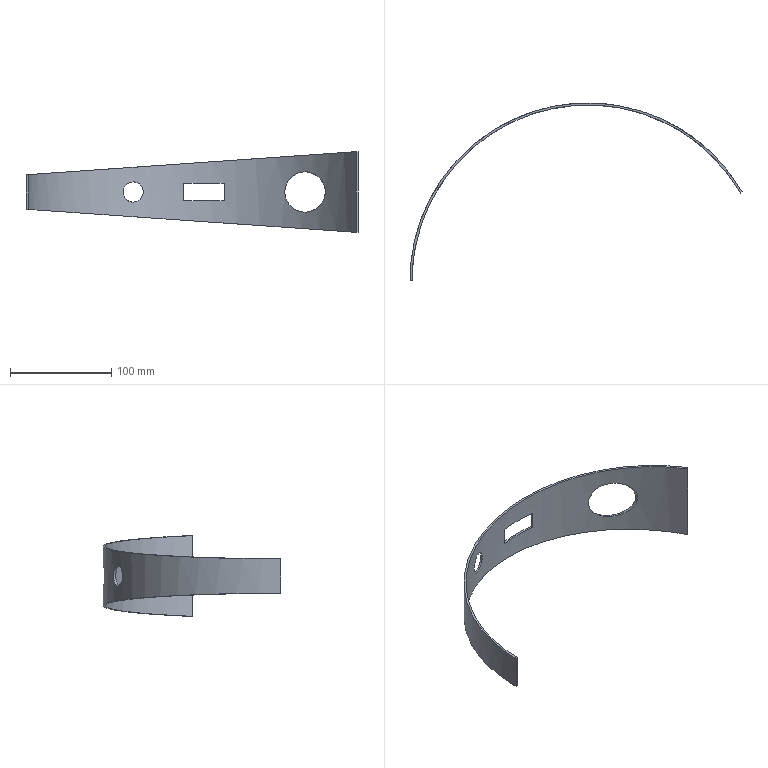Part | SolidWorks | features ICE 4, ExtruRefSurface 1, Thicken 1 | 1 solid | 14 faces | box 328.42 x 176 x 80 mm | volume 44356 mm3 | plane 8 | cylinder 6 | commonest cylinder face diameters 20 x2 40 x2 348 x1 352 x1
STEP:
#1=CARTESIAN_POINT('',(-70.,161.481,-10.));
#2=VERTEX_POINT('',#1);
#3=CARTESIAN_POINT('',(-70.,161.481,10.));
#4=VERTEX_POINT('',#3);
#5=CARTESIAN_POINT('',(-70.,161.481,-10.));
#6=CARTESIAN_POINT('',(-70.637,161.205,-10.));
#7=CARTESIAN_POINT('',(-71.263,160.929,-9.94));
#8=CARTESIAN_POINT('',(-72.494,160.378,-9.704));
#9=CARTESIAN_POINT('',(-73.101,160.102,-9.528));
#10=CARTESIAN_POINT('',(-74.285,159.556,-9.058));
#11=CARTESIAN_POINT('',(-74.849,159.292,-8.769));
#12=CARTESIAN_POINT('',(-75.652,158.912,-8.256));
#13=CARTESIAN_POINT('',(-75.912,158.787,-8.072));
#14=CARTESIAN_POINT('',(-76.419,158.544,-7.675));
#15=CARTESIAN_POINT('',(-76.666,158.425,-7.461));
#16=CARTESIAN_POINT('',(-77.375,158.08,-6.785));
#17=CARTESIAN_POINT('',(-77.8,157.871,-6.292));
#18=CARTESIAN_POINT('',(-78.368,157.59,-5.485));
#19=CARTESIAN_POINT('',(-78.545,157.502,-5.205));
#20=CARTESIAN_POINT('',(-78.874,157.337,-4.622));
#21=CARTESIAN_POINT('',(-79.027,157.26,-4.317));
#22=CARTESIAN_POINT('',(-79.433,157.056,-3.387));
#23=CARTESIAN_POINT('',(-79.64,156.95,-2.744));
#24=CARTESIAN_POINT('',(-79.853,156.842,-1.742));
#25=CARTESIAN_POINT('',(-79.908,156.814,-1.4));
#26=CARTESIAN_POINT('',(-79.981,156.777,-0.7103));
#27=CARTESIAN_POINT('',(-79.999,156.768,-0.3661));
#28=CARTESIAN_POINT('',(-80.002,156.767,0.6638));
#29=CARTESIAN_POINT('',(-79.933,156.802,1.349));
#30=CARTESIAN_POINT('',(-79.652,156.944,2.704));
#31=CARTESIAN_POINT('',(-79.446,157.049,3.352));
#32=CARTESIAN_POINT('',(-79.043,157.252,4.282));
#33=CARTESIAN_POINT('',(-78.893,157.328,4.586));
#34=CARTESIAN_POINT('',(-78.564,157.492,5.174));
#35=CARTESIAN_POINT('',(-78.386,157.58,5.457));
#36=CARTESIAN_POINT('',(-78.007,157.768,5.999));
#37=CARTESIAN_POINT('',(-77.806,157.868,6.259));
#38=CARTESIAN_POINT('',(-77.378,158.078,6.758));
#39=CARTESIAN_POINT('',(-77.152,158.189,6.997));
#40=CARTESIAN_POINT('',(-76.443,158.533,7.676));
#41=CARTESIAN_POINT('',(-75.936,158.777,8.073));
#42=CARTESIAN_POINT('',(-75.13,159.159,8.59));
#43=CARTESIAN_POINT('',(-74.853,159.29,8.749));
#44=CARTESIAN_POINT('',(-74.283,159.556,9.042));
#45=CARTESIAN_POINT('',(-73.992,159.691,9.174));
#46=CARTESIAN_POINT('',(-73.11,160.098,9.525));
#47=CARTESIAN_POINT('',(-72.506,160.373,9.701));
#48=CARTESIAN_POINT('',(-71.268,160.927,9.939));
#49=CARTESIAN_POINT('',(-70.63,161.208,10.));
#50=CARTESIAN_POINT('',(-70.,161.481,10.));
#51=B_SPLINE_CURVE_WITH_KNOTS('',3,(#5,#6,#7,#8,#9,#10,#11,#12,#13,#14,#15,#16,#17,#18,#19,#20,#21,#22,#23,#24,#25,#26,#27,#28,#29,#30,#31,#32,#33,#34,#35,#36,#37,#38,#39,#40,#41,#42,#43,#44,#45,#46,#47,#48,#49,#50),.UNSPECIFIED.,.F.,.F.,(4,2,2,2,2,2,2,2,2,2,2,2,2,2,2,2,2,2,2,2,2,2,4),(0.,0.002054,0.004107,0.006161,0.007188,0.008214,0.01027,0.01129,0.01232,0.01438,0.0154,0.01643,0.01848,0.02054,0.02156,0.02259,0.02362,0.02464,0.0267,0.02772,0.02875,0.0308,0.03286),.UNSPECIFIED.);
#52=EDGE_CURVE('',#2,#4,#51,.T.);
#53=ORIENTED_EDGE('',*,*,#52,.T.);
#54=CARTESIAN_POINT('',(-70.,159.298,10.));
#55=VERTEX_POINT('',#54);
#56=CARTESIAN_POINT('',(-70.,176.001,10.));
#57=DIRECTION('',(0.,-1.,0.));
#58=VECTOR('',#57,1000.);
#59=LINE('',#56,#58);
#60=EDGE_CURVE('',#4,#55,#59,.T.);
#61=ORIENTED_EDGE('',*,*,#60,.T.);
#62=CARTESIAN_POINT('',(-70.,159.298,-10.));
#63=VERTEX_POINT('',#62);
#64=CARTESIAN_POINT('',(-70.,159.298,10.));
#65=CARTESIAN_POINT('',(-70.629,159.022,10.));
#66=CARTESIAN_POINT('',(-71.253,158.743,9.941));
#67=CARTESIAN_POINT('',(-72.183,158.322,9.764));
#68=CARTESIAN_POINT('',(-72.493,158.18,9.69));
#69=CARTESIAN_POINT('',(-73.099,157.901,9.513));
#70=CARTESIAN_POINT('',(-73.397,157.763,9.411));
#71=CARTESIAN_POINT('',(-74.273,157.353,9.063));
#72=CARTESIAN_POINT('',(-74.836,157.086,8.776));
#73=CARTESIAN_POINT('',(-75.646,156.696,8.26));
#74=CARTESIAN_POINT('',(-75.911,156.568,8.072));
#75=CARTESIAN_POINT('',(-76.418,156.321,7.675));
#76=CARTESIAN_POINT('',(-76.662,156.202,7.465));
#77=CARTESIAN_POINT('',(-77.362,155.857,6.798));
#78=CARTESIAN_POINT('',(-77.789,155.644,6.307));
#79=CARTESIAN_POINT('',(-78.364,155.355,5.491));
#80=CARTESIAN_POINT('',(-78.544,155.264,5.206));
#81=CARTESIAN_POINT('',(-78.873,155.097,4.624));
#82=CARTESIAN_POINT('',(-79.022,155.021,4.326));
#83=CARTESIAN_POINT('',(-79.292,154.883,3.712));
#84=CARTESIAN_POINT('',(-79.411,154.822,3.397));
#85=CARTESIAN_POINT('',(-79.62,154.715,2.751));
#86=CARTESIAN_POINT('',(-79.71,154.669,2.417));
#87=CARTESIAN_POINT('',(-79.925,154.557,1.404));
#88=CARTESIAN_POINT('',(-79.998,154.52,0.7221));
#89=CARTESIAN_POINT('',(-80.001,154.518,-0.3097));
#90=CARTESIAN_POINT('',(-79.984,154.527,-0.6562));
#91=CARTESIAN_POINT('',(-79.915,154.563,-1.348));
#92=CARTESIAN_POINT('',(-79.862,154.59,-1.688));
#93=CARTESIAN_POINT('',(-79.724,154.661,-2.359));
#94=CARTESIAN_POINT('',(-79.638,154.706,-2.689));
#95=CARTESIAN_POINT('',(-79.432,154.811,-3.339));
#96=CARTESIAN_POINT('',(-79.313,154.873,-3.66));
#97=CARTESIAN_POINT('',(-78.907,155.08,-4.597));
#98=CARTESIAN_POINT('',(-78.58,155.246,-5.18));
#99=CARTESIAN_POINT('',(-78.01,155.533,-5.996));
#100=CARTESIAN_POINT('',(-77.806,155.635,-6.259));
#101=CARTESIAN_POINT('',(-77.376,155.849,-6.76));
#102=CARTESIAN_POINT('',(-77.151,155.961,-6.997));
#103=CARTESIAN_POINT('',(-76.449,156.307,-7.67));
#104=CARTESIAN_POINT('',(-75.943,156.554,-8.068));
#105=CARTESIAN_POINT('',(-74.857,157.076,-8.765));
#106=CARTESIAN_POINT('',(-74.292,157.344,-9.054));
#107=CARTESIAN_POINT('',(-73.414,157.755,-9.405));
#108=CARTESIAN_POINT('',(-73.116,157.893,-9.508));
#109=CARTESIAN_POINT('',(-72.509,158.173,-9.685));
#110=CARTESIAN_POINT('',(-72.199,158.314,-9.76));
#111=CARTESIAN_POINT('',(-71.266,158.737,-9.94));
#112=CARTESIAN_POINT('',(-70.636,159.019,-10.));
#113=CARTESIAN_POINT('',(-70.,159.298,-10.));
#114=B_SPLINE_CURVE_WITH_KNOTS('',3,(#64,#65,#66,#67,#68,#69,#70,#71,#72,#73,#74,#75,#76,#77,#78,#79,#80,#81,#82,#83,#84,#85,#86,#87,#88,#89,#90,#91,#92,#93,#94,#95,#96,#97,#98,#99,#100,#101,#102,#103,#104,#105,#106,#107,#108,#109,#110,#111,#112,#113),.UNSPECIFIED.,.F.,.F.,(4,2,2,2,2,2,2,2,2,2,2,2,2,2,2,2,2,2,2,2,2,2,2,2,4),(0.0325,0.03456,0.03558,0.03661,0.03867,0.0397,0.04072,0.04278,0.04381,0.04483,0.04586,0.04689,0.04895,0.04997,0.051,0.05203,0.05306,0.05511,0.05614,0.05717,0.05922,0.06128,0.06231,0.06334,0.06539),.UNSPECIFIED.);
#115=EDGE_CURVE('',#55,#63,#114,.T.);
#116=ORIENTED_EDGE('',*,*,#115,.T.);
#117=CARTESIAN_POINT('',(-70.,176.001,-10.));
#118=DIRECTION('',(0.,-1.,0.));
#119=VECTOR('',#118,1000.);
#120=LINE('',#117,#119);
#121=EDGE_CURVE('',#2,#63,#120,.T.);
#122=ORIENTED_EDGE('',*,*,#121,.F.);
#123=EDGE_LOOP('',(#53,#61,#116,#122));
#124=FACE_OUTER_BOUND('',#123,.T.);
#125=CARTESIAN_POINT('',(-70.,176.001,0.));
#126=DIRECTION('',(0.,-1.,0.));
#127=DIRECTION('',(0.,0.,-1.));
#128=AXIS2_PLACEMENT_3D('',#125,#126,#127);
#129=CYLINDRICAL_SURFACE('',#128,10.);
#130=ADVANCED_FACE('',(#124),#129,.F.);
#131=CARTESIAN_POINT('',(100.,144.831,-20.));
#132=VERTEX_POINT('',#131);
#133=CARTESIAN_POINT('',(100.,144.831,20.));
#134=VERTEX_POINT('',#133);
#135=CARTESIAN_POINT('',(100.,144.831,-20.));
#136=CARTESIAN_POINT('',(98.822,145.645,-20.));
#137=CARTESIAN_POINT('',(97.649,146.433,-19.897));
#138=CARTESIAN_POINT('',(95.319,147.96,-19.48));
#139=CARTESIAN_POINT('',(94.161,148.699,-19.168));
#140=CARTESIAN_POINT('',(92.726,149.593,-18.633));
#141=CARTESIAN_POINT('',(92.439,149.77,-18.518));
#142=CARTESIAN_POINT('',(91.867,150.122,-18.274));
#143=CARTESIAN_POINT('',(91.581,150.296,-18.145));
#144=CARTESIAN_POINT('',(90.733,150.811,-17.735));
#145=CARTESIAN_POINT('',(90.179,151.142,-17.434));
#146=CARTESIAN_POINT('',(88.556,152.103,-16.451));
#147=CARTESIAN_POINT('',(87.522,152.699,-15.686));
#148=CARTESIAN_POINT('',(86.059,153.526,-14.356));
#149=CARTESIAN_POINT('',(85.585,153.79,-13.88));
#150=CARTESIAN_POINT('',(84.693,154.284,-12.889));
#151=CARTESIAN_POINT('',(84.27,154.515,-12.37));
#152=CARTESIAN_POINT('',(83.475,154.946,-11.286));
#153=CARTESIAN_POINT('',(83.102,155.146,-10.721));
#154=CARTESIAN_POINT('',(82.409,155.515,-9.541));
#155=CARTESIAN_POINT('',(82.088,155.685,-8.925));
#156=CARTESIAN_POINT('',(81.215,156.143,-7.007));
#157=CARTESIAN_POINT('',(80.772,156.371,-5.68));
#158=CARTESIAN_POINT('',(80.317,156.605,-3.616));
#159=CARTESIAN_POINT('',(80.201,156.665,-2.916));
#160=CARTESIAN_POINT('',(80.082,156.725,-1.847));
#161=CARTESIAN_POINT('',(80.052,156.741,-1.488));
#162=CARTESIAN_POINT('',(80.012,156.761,-0.775));
#163=CARTESIAN_POINT('',(80.001,156.767,-0.4189));
#164=CARTESIAN_POINT('',(79.996,156.77,1.358));
#165=CARTESIAN_POINT('',(80.141,156.696,2.771));
#166=CARTESIAN_POINT('',(80.738,156.389,5.57));
#167=CARTESIAN_POINT('',(81.177,156.162,6.903));
#168=CARTESIAN_POINT('',(81.889,155.789,8.492));
#169=CARTESIAN_POINT('',(82.039,155.71,8.805));
#170=CARTESIAN_POINT('',(82.357,155.542,9.425));
#171=CARTESIAN_POINT('',(82.524,155.454,9.732));
#172=CARTESIAN_POINT('',(83.045,155.176,10.631));
#173=CARTESIAN_POINT('',(83.419,154.976,11.204));
#174=CARTESIAN_POINT('',(84.215,154.545,12.3));
#175=CARTESIAN_POINT('',(84.637,154.314,12.823));
#176=CARTESIAN_POINT('',(85.306,153.945,13.572));
#177=CARTESIAN_POINT('',(85.535,153.818,13.815));
#178=CARTESIAN_POINT('',(86.004,153.556,14.29));
#179=CARTESIAN_POINT('',(86.244,153.421,14.522));
#180=CARTESIAN_POINT('',(87.463,152.734,15.638));
#181=CARTESIAN_POINT('',(88.497,152.138,16.41));
#182=CARTESIAN_POINT('',(90.125,151.175,17.404));
#183=CARTESIAN_POINT('',(90.683,150.841,17.708));
#184=CARTESIAN_POINT('',(91.815,150.155,18.259));
#185=CARTESIAN_POINT('',(92.386,149.804,18.504));
#186=CARTESIAN_POINT('',(94.112,148.731,19.153));
#187=CARTESIAN_POINT('',(95.279,147.986,19.472));
#188=CARTESIAN_POINT('',(97.052,146.824,19.791));
#189=CARTESIAN_POINT('',(97.648,146.429,19.87));
#190=CARTESIAN_POINT('',(98.829,145.634,19.974));
#191=CARTESIAN_POINT('',(99.416,145.234,20.));
#192=CARTESIAN_POINT('',(100.,144.831,20.));
#193=B_SPLINE_CURVE_WITH_KNOTS('',3,(#135,#136,#137,#138,#139,#140,#141,#142,#143,#144,#145,#146,#147,#148,#149,#150,#151,#152,#153,#154,#155,#156,#157,#158,#159,#160,#161,#162,#163,#164,#165,#166,#167,#168,#169,#170,#171,#172,#173,#174,#175,#176,#177,#178,#179,#180,#181,#182,#183,#184,#185,#186,#187,#188,#189,#190,#191,#192),.UNSPECIFIED.,.F.,.F.,(4,2,2,2,2,2,2,2,2,2,2,2,2,2,2,2,2,2,2,2,2,2,2,2,2,2,2,2,4),(0.,0.004223,0.008446,0.009502,0.01056,0.01267,0.01689,0.019,0.02112,0.02323,0.02534,0.02956,0.03167,0.03273,0.03379,0.03801,0.04223,0.04329,0.04434,0.04646,0.04857,0.04962,0.05068,0.0549,0.05701,0.05912,0.06335,0.06546,0.06757),.UNSPECIFIED.);
#194=EDGE_CURVE('',#132,#134,#193,.T.);
#195=ORIENTED_EDGE('',*,*,#194,.T.);
#196=CARTESIAN_POINT('',(100.,142.394,20.));
#197=VERTEX_POINT('',#196);
#198=CARTESIAN_POINT('',(100.,176.001,20.));
#199=DIRECTION('',(0.,-1.,0.));
#200=VECTOR('',#199,1000.);
#201=LINE('',#198,#200);
#202=EDGE_CURVE('',#134,#197,#201,.T.);
#203=ORIENTED_EDGE('',*,*,#202,.T.);
#204=CARTESIAN_POINT('',(100.,142.394,-20.));
#205=VERTEX_POINT('',#204);
#206=CARTESIAN_POINT('',(100.,142.394,20.));
#207=CARTESIAN_POINT('',(98.843,143.206,20.));
#208=CARTESIAN_POINT('',(97.676,144.005,19.9));
#209=CARTESIAN_POINT('',(95.911,145.181,19.587));
#210=CARTESIAN_POINT('',(95.319,145.57,19.454));
#211=CARTESIAN_POINT('',(94.153,146.327,19.136));
#212=CARTESIAN_POINT('',(93.576,146.697,18.95));
#213=CARTESIAN_POINT('',(91.861,147.782,18.31));
#214=CARTESIAN_POINT('',(90.741,148.471,17.774));
#215=CARTESIAN_POINT('',(89.379,149.29,16.95));
#216=CARTESIAN_POINT('',(89.107,149.452,16.777));
#217=CARTESIAN_POINT('',(88.574,149.769,16.418));
#218=CARTESIAN_POINT('',(88.311,149.924,16.232));
#219=CARTESIAN_POINT('',(87.537,150.378,15.655));
#220=CARTESIAN_POINT('',(87.038,150.668,15.245));
#221=CARTESIAN_POINT('',(85.594,151.496,13.934));
#222=CARTESIAN_POINT('',(84.702,151.995,12.955));
#223=CARTESIAN_POINT('',(83.691,152.551,11.582));
#224=CARTESIAN_POINT('',(83.494,152.659,11.299));
#225=CARTESIAN_POINT('',(83.116,152.865,10.726));
#226=CARTESIAN_POINT('',(82.934,152.964,10.434));
#227=CARTESIAN_POINT('',(82.412,153.246,9.547));
#228=CARTESIAN_POINT('',(82.094,153.417,8.936));
#229=CARTESIAN_POINT('',(81.52,153.722,7.679));
#230=CARTESIAN_POINT('',(81.264,153.858,7.032));
#231=CARTESIAN_POINT('',(80.928,154.035,6.032));
#232=CARTESIAN_POINT('',(80.824,154.089,5.693));
#233=CARTESIAN_POINT('',(80.634,154.189,5.007));
#234=CARTESIAN_POINT('',(80.547,154.234,4.659));
#235=CARTESIAN_POINT('',(80.163,154.434,2.921));
#236=CARTESIAN_POINT('',(80.006,154.515,1.511));
#237=CARTESIAN_POINT('',(79.997,154.52,-0.6317));
#238=CARTESIAN_POINT('',(80.033,154.501,-1.356));
#239=CARTESIAN_POINT('',(80.181,154.425,-2.779));
#240=CARTESIAN_POINT('',(80.293,154.367,-3.481));
#241=CARTESIAN_POINT('',(80.588,154.213,-4.865));
#242=CARTESIAN_POINT('',(80.772,154.117,-5.547));
#243=CARTESIAN_POINT('',(81.211,153.886,-6.891));
#244=CARTESIAN_POINT('',(81.469,153.75,-7.555));
#245=CARTESIAN_POINT('',(82.327,153.293,-9.467));
#246=CARTESIAN_POINT('',(83.02,152.92,-10.656));
#247=CARTESIAN_POINT('',(84.025,152.368,-12.038));
#248=CARTESIAN_POINT('',(84.233,152.253,-12.309));
#249=CARTESIAN_POINT('',(84.659,152.016,-12.837));
#250=CARTESIAN_POINT('',(84.878,151.894,-13.093));
#251=CARTESIAN_POINT('',(85.547,151.519,-13.841));
#252=CARTESIAN_POINT('',(86.013,151.255,-14.311));
#253=CARTESIAN_POINT('',(86.982,150.7,-15.197));
#254=CARTESIAN_POINT('',(87.484,150.409,-15.613));
#255=CARTESIAN_POINT('',(88.524,149.799,-16.393));
#256=CARTESIAN_POINT('',(89.061,149.481,-16.755));
#257=CARTESIAN_POINT('',(90.69,148.502,-17.746));
#258=CARTESIAN_POINT('',(91.812,147.812,-18.289));
#259=CARTESIAN_POINT('',(93.541,146.719,-18.938));
#260=CARTESIAN_POINT('',(94.127,146.344,-19.128));
#261=CARTESIAN_POINT('',(95.299,145.584,-19.449));
#262=CARTESIAN_POINT('',(95.886,145.198,-19.581));
#263=CARTESIAN_POINT('',(97.06,144.416,-19.792));
#264=CARTESIAN_POINT('',(97.647,144.019,-19.87));
#265=CARTESIAN_POINT('',(98.823,143.215,-19.974));
#266=CARTESIAN_POINT('',(99.413,142.806,-20.));
#267=CARTESIAN_POINT('',(100.,142.394,-20.));
#268=B_SPLINE_CURVE_WITH_KNOTS('',3,(#206,#207,#208,#209,#210,#211,#212,#213,#214,#215,#216,#217,#218,#219,#220,#221,#222,#223,#224,#225,#226,#227,#228,#229,#230,#231,#232,#233,#234,#235,#236,#237,#238,#239,#240,#241,#242,#243,#244,#245,#246,#247,#248,#249,#250,#251,#252,#253,#254,#255,#256,#257,#258,#259,#260,#261,#262,#263,#264,#265,#266,#267),.UNSPECIFIED.,.F.,.F.,(4,2,2,2,2,2,2,2,2,2,2,2,2,2,2,2,2,2,2,2,2,2,2,2,2,2,2,2,2,2,4),(0.07152,0.07577,0.07789,0.08001,0.08425,0.08531,0.08637,0.08849,0.09273,0.09379,0.09485,0.09697,0.0991,0.1002,0.1012,0.1055,0.1076,0.1097,0.1118,0.1139,0.1182,0.1192,0.1203,0.1224,0.1245,0.1267,0.1309,0.133,0.1352,0.1373,0.1394),.UNSPECIFIED.);
#269=EDGE_CURVE('',#197,#205,#268,.T.);
#270=ORIENTED_EDGE('',*,*,#269,.T.);
#271=CARTESIAN_POINT('',(100.,176.001,-20.));
#272=DIRECTION('',(0.,-1.,0.));
#273=VECTOR('',#272,1000.);
#274=LINE('',#271,#273);
#275=EDGE_CURVE('',#132,#205,#274,.T.);
#276=ORIENTED_EDGE('',*,*,#275,.F.);
#277=EDGE_LOOP('',(#195,#203,#270,#276));
#278=FACE_OUTER_BOUND('',#277,.T.);
#279=CARTESIAN_POINT('',(100.,176.001,0.));
#280=DIRECTION('',(0.,-1.,0.));
#281=DIRECTION('',(0.,0.,-1.));
#282=AXIS2_PLACEMENT_3D('',#279,#280,#281);
#283=CYLINDRICAL_SURFACE('',#282,20.);
#284=ADVANCED_FACE('',(#278),#283,.F.);
#285=ORIENTED_EDGE('',*,*,#194,.F.);
#286=CARTESIAN_POINT('',(100.,144.831,20.));
#287=CARTESIAN_POINT('',(101.225,143.985,20.));
#288=CARTESIAN_POINT('',(102.436,143.126,19.888));
#289=CARTESIAN_POINT('',(104.232,141.818,19.557));
#290=CARTESIAN_POINT('',(104.828,141.377,19.418));
#291=CARTESIAN_POINT('',(105.996,140.504,19.09));
#292=CARTESIAN_POINT('',(106.569,140.07,18.9));
#293=CARTESIAN_POINT('',(108.261,138.772,18.254));
#294=CARTESIAN_POINT('',(109.35,137.915,17.723));
#295=CARTESIAN_POINT('',(110.924,136.646,16.764));
#296=CARTESIAN_POINT('',(111.441,136.225,16.416));
#297=CARTESIAN_POINT('',(112.446,135.397,15.668));
#298=CARTESIAN_POINT('',(112.932,134.992,15.27));
#299=CARTESIAN_POINT('',(114.338,133.807,14.001));
#300=CARTESIAN_POINT('',(115.208,133.057,13.057));
#301=CARTESIAN_POINT('',(116.402,132.011,11.464));
#302=CARTESIAN_POINT('',(116.781,131.675,10.902));
#303=CARTESIAN_POINT('',(117.483,131.05,9.737));
#304=CARTESIAN_POINT('',(117.807,130.758,9.132));
#305=CARTESIAN_POINT('',(118.399,130.223,7.873));
#306=CARTESIAN_POINT('',(118.666,129.979,7.218));
#307=CARTESIAN_POINT('',(119.02,129.655,6.195));
#308=CARTESIAN_POINT('',(119.13,129.554,5.847));
#309=CARTESIAN_POINT('',(119.33,129.369,5.147));
#310=CARTESIAN_POINT('',(119.42,129.286,4.794));
#311=CARTESIAN_POINT('',(119.664,129.061,3.724));
#312=CARTESIAN_POINT('',(119.788,128.945,2.998));
#313=CARTESIAN_POINT('',(119.956,128.789,1.516));
#314=CARTESIAN_POINT('',(120.,128.748,0.7568));
#315=CARTESIAN_POINT('',(120.,128.748,-0.7399));
#316=CARTESIAN_POINT('',(119.959,128.786,-1.483));
#317=CARTESIAN_POINT('',(119.835,128.901,-2.59));
#318=CARTESIAN_POINT('',(119.784,128.949,-2.957));
#319=CARTESIAN_POINT('',(119.66,129.064,-3.69));
#320=CARTESIAN_POINT('',(119.588,129.131,-4.056));
#321=CARTESIAN_POINT('',(119.181,129.508,-5.855));
#322=CARTESIAN_POINT('',(118.709,129.941,-7.208));
#323=CARTESIAN_POINT('',(117.513,131.024,-9.762));
#324=CARTESIAN_POINT('',(116.81,131.653,-10.916));
#325=CARTESIAN_POINT('',(115.625,132.692,-12.501));
#326=CARTESIAN_POINT('',(115.208,133.054,-13.005));
#327=CARTESIAN_POINT('',(114.331,133.809,-13.966));
#328=CARTESIAN_POINT('',(113.874,134.198,-14.419));
#329=CARTESIAN_POINT('',(112.466,135.384,-15.691));
#330=CARTESIAN_POINT('',(111.472,136.205,-16.429));
#331=CARTESIAN_POINT('',(109.902,137.47,-17.387));
#332=CARTESIAN_POINT('',(109.366,137.897,-17.682));
#333=CARTESIAN_POINT('',(108.265,138.763,-18.222));
#334=CARTESIAN_POINT('',(107.703,139.199,-18.467));
#335=CARTESIAN_POINT('',(106.003,140.504,-19.117));
#336=CARTESIAN_POINT('',(104.841,141.374,-19.443));
#337=CARTESIAN_POINT('',(103.057,142.674,-19.774));
#338=CARTESIAN_POINT('',(102.455,143.107,-19.858));
#339=CARTESIAN_POINT('',(101.236,143.972,-19.971));
#340=CARTESIAN_POINT('',(100.618,144.404,-20.));
#341=CARTESIAN_POINT('',(100.,144.831,-20.));
#342=B_SPLINE_CURVE_WITH_KNOTS('',3,(#286,#287,#288,#289,#290,#291,#292,#293,#294,#295,#296,#297,#298,#299,#300,#301,#302,#303,#304,#305,#306,#307,#308,#309,#310,#311,#312,#313,#314,#315,#316,#317,#318,#319,#320,#321,#322,#323,#324,#325,#326,#327,#328,#329,#330,#331,#332,#333,#334,#335,#336,#337,#338,#339,#340,#341),.UNSPECIFIED.,.F.,.F.,(4,2,2,2,2,2,2,2,2,2,2,2,2,2,2,2,2,2,2,2,2,2,2,2,2,2,2,4),(0.06757,0.072,0.07421,0.07643,0.08086,0.08307,0.08529,0.08971,0.09193,0.09414,0.09636,0.09746,0.09857,0.1008,0.103,0.1052,0.1063,0.1074,0.1119,0.1163,0.1185,0.1207,0.1251,0.1274,0.1296,0.134,0.1362,0.1384),.UNSPECIFIED.);
#343=EDGE_CURVE('',#134,#132,#342,.T.);
#344=ORIENTED_EDGE('',*,*,#343,.F.);
#345=EDGE_LOOP('',(#285,#344));
#346=FACE_BOUND('',#345,.T.);
#347=CARTESIAN_POINT('',(-176.,0.,-17.035));
#348=VERTEX_POINT('',#347);
#349=CARTESIAN_POINT('',(152.42,88.,-40.));
#350=VERTEX_POINT('',#349);
#351=CARTESIAN_POINT('',(-176.,0.,-17.035));
#352=CARTESIAN_POINT('',(-176.,224.036,-17.035));
#353=CARTESIAN_POINT('',(40.402,282.021,-32.167));
#354=CARTESIAN_POINT('',(152.42,88.,-40.));
#355=(BOUNDED_CURVE()B_SPLINE_CURVE(3,(#351,#352,#353,#354),.UNSPECIFIED.,.F.,.F.)B_SPLINE_CURVE_WITH_KNOTS((4,4),(0.,2.618),.UNSPECIFIED.)CURVE()GEOMETRIC_REPRESENTATION_ITEM()RATIONAL_B_SPLINE_CURVE((1.,0.5059,0.5059,1.))REPRESENTATION_ITEM(''));
#356=EDGE_CURVE('',#348,#350,#355,.T.);
#357=ORIENTED_EDGE('',*,*,#356,.F.);
#358=CARTESIAN_POINT('',(-176.,0.,17.035));
#359=VERTEX_POINT('',#358);
#360=CARTESIAN_POINT('',(-176.,0.,-40.));
#361=DIRECTION('',(0.,0.,1.));
#362=VECTOR('',#361,1000.);
#363=LINE('',#360,#362);
#364=EDGE_CURVE('',#348,#359,#363,.T.);
#365=ORIENTED_EDGE('',*,*,#364,.T.);
#366=CARTESIAN_POINT('',(152.42,88.,40.));
#367=VERTEX_POINT('',#366);
#368=CARTESIAN_POINT('',(152.42,88.,40.));
#369=CARTESIAN_POINT('',(40.402,282.021,32.167));
#370=CARTESIAN_POINT('',(-176.,224.036,17.035));
#371=CARTESIAN_POINT('',(-176.,0.,17.035));
#372=(BOUNDED_CURVE()B_SPLINE_CURVE(3,(#368,#369,#370,#371),.UNSPECIFIED.,.F.,.F.)B_SPLINE_CURVE_WITH_KNOTS((4,4),(0.5236,3.142),.UNSPECIFIED.)CURVE()GEOMETRIC_REPRESENTATION_ITEM()RATIONAL_B_SPLINE_CURVE((1.,0.5059,0.5059,1.))REPRESENTATION_ITEM(''));
#373=EDGE_CURVE('',#367,#359,#372,.T.);
#374=ORIENTED_EDGE('',*,*,#373,.F.);
#375=CARTESIAN_POINT('',(152.42,88.,-40.));
#376=DIRECTION('',(0.,0.,1.));
#377=VECTOR('',#376,1000.);
#378=LINE('',#375,#377);
#379=EDGE_CURVE('',#350,#367,#378,.T.);
#380=ORIENTED_EDGE('',*,*,#379,.F.);
#381=EDGE_LOOP('',(#357,#365,#374,#380));
#382=FACE_OUTER_BOUND('',#381,.T.);
#383=CARTESIAN_POINT('',(20.,174.86,-8.5));
#384=VERTEX_POINT('',#383);
#385=CARTESIAN_POINT('',(-20.,174.86,-8.5));
#386=VERTEX_POINT('',#385);
#387=CARTESIAN_POINT('',(0.,0.,-8.5));
#388=DIRECTION('',(0.,0.,1.));
#389=DIRECTION('',(1.,0.,0.));
#390=AXIS2_PLACEMENT_3D('',#387,#388,#389);
#391=CIRCLE('',#390,176.);
#392=EDGE_CURVE('',#384,#386,#391,.T.);
#393=ORIENTED_EDGE('',*,*,#392,.F.);
#394=CARTESIAN_POINT('',(20.,174.86,8.5));
#395=VERTEX_POINT('',#394);
#396=CARTESIAN_POINT('',(20.,174.86,-40.));
#397=DIRECTION('',(0.,0.,-1.));
#398=VECTOR('',#397,1000.);
#399=LINE('',#396,#398);
#400=EDGE_CURVE('',#395,#384,#399,.T.);
#401=ORIENTED_EDGE('',*,*,#400,.F.);
#402=CARTESIAN_POINT('',(-20.,174.86,8.5));
#403=VERTEX_POINT('',#402);
#404=CARTESIAN_POINT('',(0.,0.,8.5));
#405=DIRECTION('',(0.,0.,-1.));
#406=DIRECTION('',(-1.,0.,0.));
#407=AXIS2_PLACEMENT_3D('',#404,#405,#406);
#408=CIRCLE('',#407,176.);
#409=EDGE_CURVE('',#403,#395,#408,.T.);
#410=ORIENTED_EDGE('',*,*,#409,.F.);
#411=CARTESIAN_POINT('',(-20.,174.86,-40.));
#412=DIRECTION('',(0.,0.,1.));
#413=VECTOR('',#412,1000.);
#414=LINE('',#411,#413);
#415=EDGE_CURVE('',#386,#403,#414,.T.);
#416=ORIENTED_EDGE('',*,*,#415,.F.);
#417=EDGE_LOOP('',(#393,#401,#410,#416));
#418=FACE_BOUND('',#417,.T.);
#419=ORIENTED_EDGE('',*,*,#52,.F.);
#420=CARTESIAN_POINT('',(-70.,161.481,10.));
#421=CARTESIAN_POINT('',(-69.378,161.75,10.));
#422=CARTESIAN_POINT('',(-68.759,162.014,9.943));
#423=CARTESIAN_POINT('',(-67.833,162.403,9.767));
#424=CARTESIAN_POINT('',(-67.524,162.532,9.694));
#425=CARTESIAN_POINT('',(-66.913,162.784,9.517));
#426=CARTESIAN_POINT('',(-66.614,162.907,9.414));
#427=CARTESIAN_POINT('',(-65.731,163.266,9.065));
#428=CARTESIAN_POINT('',(-65.164,163.493,8.777));
#429=CARTESIAN_POINT('',(-64.348,163.815,8.256));
#430=CARTESIAN_POINT('',(-64.081,163.92,8.066));
#431=CARTESIAN_POINT('',(-63.567,164.12,7.663));
#432=CARTESIAN_POINT('',(-63.321,164.215,7.45));
#433=CARTESIAN_POINT('',(-62.615,164.486,6.774));
#434=CARTESIAN_POINT('',(-62.186,164.648,6.277));
#435=CARTESIAN_POINT('',(-61.613,164.863,5.456));
#436=CARTESIAN_POINT('',(-61.433,164.93,5.169));
#437=CARTESIAN_POINT('',(-61.107,165.052,4.585));
#438=CARTESIAN_POINT('',(-60.958,165.106,4.285));
#439=CARTESIAN_POINT('',(-60.692,165.204,3.671));
#440=CARTESIAN_POINT('',(-60.574,165.248,3.357));
#441=CARTESIAN_POINT('',(-60.369,165.323,2.713));
#442=CARTESIAN_POINT('',(-60.282,165.355,2.382));
#443=CARTESIAN_POINT('',(-60.072,165.431,1.38));
#444=CARTESIAN_POINT('',(-60.002,165.456,0.7065));
#445=CARTESIAN_POINT('',(-59.999,165.457,-0.3118));
#446=CARTESIAN_POINT('',(-60.015,165.451,-0.6534));
#447=CARTESIAN_POINT('',(-60.084,165.427,-1.336));
#448=CARTESIAN_POINT('',(-60.135,165.408,-1.673));
#449=CARTESIAN_POINT('',(-60.339,165.334,-2.667));
#450=CARTESIAN_POINT('',(-60.54,165.26,-3.311));
#451=CARTESIAN_POINT('',(-61.075,165.063,-4.561));
#452=CARTESIAN_POINT('',(-61.4,164.943,-5.146));
#453=CARTESIAN_POINT('',(-61.967,164.731,-5.965));
#454=CARTESIAN_POINT('',(-62.169,164.654,-6.228));
#455=CARTESIAN_POINT('',(-62.6,164.491,-6.735));
#456=CARTESIAN_POINT('',(-62.828,164.404,-6.976));
#457=CARTESIAN_POINT('',(-63.536,164.132,-7.659));
#458=CARTESIAN_POINT('',(-64.046,163.934,-8.06));
#459=CARTESIAN_POINT('',(-64.863,163.612,-8.586));
#460=CARTESIAN_POINT('',(-65.146,163.5,-8.749));
#461=CARTESIAN_POINT('',(-65.717,163.271,-9.042));
#462=CARTESIAN_POINT('',(-66.007,163.154,-9.174));
#463=CARTESIAN_POINT('',(-66.891,162.794,-9.526));
#464=CARTESIAN_POINT('',(-67.499,162.543,-9.703));
#465=CARTESIAN_POINT('',(-68.744,162.021,-9.941));
#466=CARTESIAN_POINT('',(-69.371,161.753,-10.));
#467=CARTESIAN_POINT('',(-70.,161.481,-10.));
#468=B_SPLINE_CURVE_WITH_KNOTS('',3,(#420,#421,#422,#423,#424,#425,#426,#427,#428,#429,#430,#431,#432,#433,#434,#435,#436,#437,#438,#439,#440,#441,#442,#443,#444,#445,#446,#447,#448,#449,#450,#451,#452,#453,#454,#455,#456,#457,#458,#459,#460,#461,#462,#463,#464,#465,#466,#467),.UNSPECIFIED.,.F.,.F.,(4,2,2,2,2,2,2,2,2,2,2,2,2,2,2,2,2,2,2,2,2,2,2,4),(0.03286,0.03488,0.0359,0.03691,0.03894,0.03995,0.04096,0.04299,0.044,0.04502,0.04603,0.04704,0.04907,0.05008,0.05109,0.05312,0.05515,0.05616,0.05717,0.0592,0.06021,0.06123,0.06325,0.06528),.UNSPECIFIED.);
#469=EDGE_CURVE('',#4,#2,#468,.T.);
#470=ORIENTED_EDGE('',*,*,#469,.F.);
#471=EDGE_LOOP('',(#419,#470));
#472=FACE_BOUND('',#471,.T.);
#473=CARTESIAN_POINT('',(0.,0.,-40.));
#474=DIRECTION('',(0.,0.,1.));
#475=DIRECTION('',(1.,0.,0.));
#476=AXIS2_PLACEMENT_3D('',#473,#474,#475);
#477=CYLINDRICAL_SURFACE('',#476,176.);
#478=ADVANCED_FACE('',(#346,#382,#418,#472),#477,.T.);
#479=CARTESIAN_POINT('',(100.,142.394,-20.));
#480=CARTESIAN_POINT('',(101.237,141.525,-20.));
#481=CARTESIAN_POINT('',(102.447,140.652,-19.886));
#482=CARTESIAN_POINT('',(104.815,138.896,-19.449));
#483=CARTESIAN_POINT('',(105.974,138.013,-19.125));
#484=CARTESIAN_POINT('',(107.675,136.684,-18.479));
#485=CARTESIAN_POINT('',(108.238,136.239,-18.235));
#486=CARTESIAN_POINT('',(109.333,135.361,-17.699));
#487=CARTESIAN_POINT('',(109.868,134.928,-17.407));
#488=CARTESIAN_POINT('',(111.432,133.644,-16.456));
#489=CARTESIAN_POINT('',(112.423,132.81,-15.724));
#490=CARTESIAN_POINT('',(113.828,131.604,-14.463));
#491=CARTESIAN_POINT('',(114.283,131.209,-14.015));
#492=CARTESIAN_POINT('',(115.162,130.438,-13.058));
#493=CARTESIAN_POINT('',(115.584,130.064,-12.553));
#494=CARTESIAN_POINT('',(116.776,128.998,-10.969));
#495=CARTESIAN_POINT('',(117.482,128.353,-9.816));
#496=CARTESIAN_POINT('',(118.235,127.658,-8.223));
#497=CARTESIAN_POINT('',(118.378,127.525,-7.897));
#498=CARTESIAN_POINT('',(118.647,127.275,-7.239));
#499=CARTESIAN_POINT('',(118.774,127.157,-6.905));
#500=CARTESIAN_POINT('',(119.127,126.826,-5.888));
#501=CARTESIAN_POINT('',(119.328,126.636,-5.192));
#502=CARTESIAN_POINT('',(119.658,126.325,-3.756));
#503=CARTESIAN_POINT('',(119.786,126.203,-3.011));
#504=CARTESIAN_POINT('',(119.956,126.042,-1.525));
#505=CARTESIAN_POINT('',(119.999,126.001,-0.779));
#506=CARTESIAN_POINT('',(120.001,125.999,0.717));
#507=CARTESIAN_POINT('',(119.96,126.038,1.469));
#508=CARTESIAN_POINT('',(119.792,126.197,2.971));
#509=CARTESIAN_POINT('',(119.668,126.316,3.705));
#510=CARTESIAN_POINT('',(119.343,126.623,5.139));
#511=CARTESIAN_POINT('',(119.142,126.812,5.839));
#512=CARTESIAN_POINT('',(118.788,127.144,6.867));
#513=CARTESIAN_POINT('',(118.66,127.263,7.205));
#514=CARTESIAN_POINT('',(118.392,127.512,7.865));
#515=CARTESIAN_POINT('',(118.251,127.643,8.188));
#516=CARTESIAN_POINT('',(117.508,128.329,9.768));
#517=CARTESIAN_POINT('',(116.805,128.972,10.926));
#518=CARTESIAN_POINT('',(115.203,130.405,13.063));
#519=CARTESIAN_POINT('',(114.33,131.172,14.008));
#520=CARTESIAN_POINT('',(112.927,132.378,15.274));
#521=CARTESIAN_POINT('',(112.444,132.789,15.67));
#522=CARTESIAN_POINT('',(111.446,133.627,16.413));
#523=CARTESIAN_POINT('',(110.93,134.056,16.761));
#524=CARTESIAN_POINT('',(109.347,135.356,17.725));
#525=CARTESIAN_POINT('',(108.254,136.232,18.258));
#526=CARTESIAN_POINT('',(106.559,137.556,18.903));
#527=CARTESIAN_POINT('',(105.985,137.999,19.093));
#528=CARTESIAN_POINT('',(104.818,138.887,19.42));
#529=CARTESIAN_POINT('',(104.223,139.335,19.559));
#530=CARTESIAN_POINT('',(102.427,140.666,19.889));
#531=CARTESIAN_POINT('',(101.219,141.538,20.));
#532=CARTESIAN_POINT('',(100.,142.394,20.));
#533=B_SPLINE_CURVE_WITH_KNOTS('',3,(#479,#480,#481,#482,#483,#484,#485,#486,#487,#488,#489,#490,#491,#492,#493,#494,#495,#496,#497,#498,#499,#500,#501,#502,#503,#504,#505,#506,#507,#508,#509,#510,#511,#512,#513,#514,#515,#516,#517,#518,#519,#520,#521,#522,#523,#524,#525,#526,#527,#528,#529,#530,#531,#532),.UNSPECIFIED.,.F.,.F.,(4,2,2,2,2,2,2,2,2,2,2,2,2,2,2,2,2,2,2,2,2,2,2,2,2,2,4),(0.,0.00447,0.00894,0.01118,0.01341,0.01788,0.02012,0.02235,0.02682,0.02794,0.02906,0.03129,0.03353,0.03576,0.038,0.04023,0.04247,0.04358,0.0447,0.04917,0.05364,0.05588,0.05811,0.06258,0.06482,0.06705,0.07152),.UNSPECIFIED.);
#534=EDGE_CURVE('',#205,#197,#533,.T.);
#535=ORIENTED_EDGE('',*,*,#534,.F.);
#536=ORIENTED_EDGE('',*,*,#269,.F.);
#537=EDGE_LOOP('',(#535,#536));
#538=FACE_BOUND('',#537,.T.);
#539=CARTESIAN_POINT('',(-174.,0.,-17.174));
#540=VERTEX_POINT('',#539);
#541=CARTESIAN_POINT('',(-174.,0.,17.174));
#542=VERTEX_POINT('',#541);
#543=CARTESIAN_POINT('',(-174.,0.,-40.));
#544=DIRECTION('',(0.,0.,1.));
#545=VECTOR('',#544,1000.);
#546=LINE('',#543,#545);
#547=EDGE_CURVE('',#540,#542,#546,.T.);
#548=ORIENTED_EDGE('',*,*,#547,.F.);
#549=CARTESIAN_POINT('',(150.688,87.,-39.879));
#550=VERTEX_POINT('',#549);
#551=CARTESIAN_POINT('',(-174.,0.,-17.174));
#552=CARTESIAN_POINT('',(-174.,221.49,-17.174));
#553=CARTESIAN_POINT('',(39.943,278.816,-32.135));
#554=CARTESIAN_POINT('',(150.688,87.,-39.879));
#555=(BOUNDED_CURVE()B_SPLINE_CURVE(3,(#551,#552,#553,#554),.UNSPECIFIED.,.F.,.F.)B_SPLINE_CURVE_WITH_KNOTS((4,4),(0.,2.618),.UNSPECIFIED.)CURVE()GEOMETRIC_REPRESENTATION_ITEM()RATIONAL_B_SPLINE_CURVE((1.,0.5059,0.5059,1.))REPRESENTATION_ITEM(''));
#556=EDGE_CURVE('',#540,#550,#555,.T.);
#557=ORIENTED_EDGE('',*,*,#556,.T.);
#558=CARTESIAN_POINT('',(150.688,87.,39.879));
#559=VERTEX_POINT('',#558);
#560=CARTESIAN_POINT('',(150.688,87.,-40.));
#561=DIRECTION('',(0.,0.,1.));
#562=VECTOR('',#561,1000.);
#563=LINE('',#560,#562);
#564=EDGE_CURVE('',#550,#559,#563,.T.);
#565=ORIENTED_EDGE('',*,*,#564,.T.);
#566=CARTESIAN_POINT('',(150.688,87.,39.879));
#567=CARTESIAN_POINT('',(39.943,278.816,32.135));
#568=CARTESIAN_POINT('',(-174.,221.49,17.174));
#569=CARTESIAN_POINT('',(-174.,0.,17.174));
#570=(BOUNDED_CURVE()B_SPLINE_CURVE(3,(#566,#567,#568,#569),.UNSPECIFIED.,.F.,.F.)B_SPLINE_CURVE_WITH_KNOTS((4,4),(0.5236,3.142),.UNSPECIFIED.)CURVE()GEOMETRIC_REPRESENTATION_ITEM()RATIONAL_B_SPLINE_CURVE((1.,0.5059,0.5059,1.))REPRESENTATION_ITEM(''));
#571=EDGE_CURVE('',#559,#542,#570,.T.);
#572=ORIENTED_EDGE('',*,*,#571,.T.);
#573=EDGE_LOOP('',(#548,#557,#565,#572));
#574=FACE_OUTER_BOUND('',#573,.T.);
#575=CARTESIAN_POINT('',(20.,172.847,-8.5));
#576=VERTEX_POINT('',#575);
#577=CARTESIAN_POINT('',(20.,172.847,8.5));
#578=VERTEX_POINT('',#577);
#579=CARTESIAN_POINT('',(20.,172.847,-40.));
#580=DIRECTION('',(0.,0.,1.));
#581=VECTOR('',#580,1000.);
#582=LINE('',#579,#581);
#583=EDGE_CURVE('',#576,#578,#582,.T.);
#584=ORIENTED_EDGE('',*,*,#583,.F.);
#585=CARTESIAN_POINT('',(-20.,172.847,-8.5));
#586=VERTEX_POINT('',#585);
#587=CARTESIAN_POINT('',(0.,0.,-8.5));
#588=DIRECTION('',(0.,0.,-1.));
#589=DIRECTION('',(1.,0.,0.));
#590=AXIS2_PLACEMENT_3D('',#587,#588,#589);
#591=CIRCLE('',#590,174.);
#592=EDGE_CURVE('',#586,#576,#591,.T.);
#593=ORIENTED_EDGE('',*,*,#592,.F.);
#594=CARTESIAN_POINT('',(-20.,172.847,8.5));
#595=VERTEX_POINT('',#594);
#596=CARTESIAN_POINT('',(-20.,172.847,-40.));
#597=DIRECTION('',(0.,0.,-1.));
#598=VECTOR('',#597,1000.);
#599=LINE('',#596,#598);
#600=EDGE_CURVE('',#595,#586,#599,.T.);
#601=ORIENTED_EDGE('',*,*,#600,.F.);
#602=CARTESIAN_POINT('',(0.,0.,8.5));
#603=DIRECTION('',(0.,0.,1.));
#604=DIRECTION('',(-1.,0.,0.));
#605=AXIS2_PLACEMENT_3D('',#602,#603,#604);
#606=CIRCLE('',#605,174.);
#607=EDGE_CURVE('',#578,#595,#606,.T.);
#608=ORIENTED_EDGE('',*,*,#607,.F.);
#609=EDGE_LOOP('',(#584,#593,#601,#608));
#610=FACE_BOUND('',#609,.T.);
#611=CARTESIAN_POINT('',(-70.,159.298,-10.));
#612=CARTESIAN_POINT('',(-69.372,159.575,-10.));
#613=CARTESIAN_POINT('',(-68.75,159.843,-9.941));
#614=CARTESIAN_POINT('',(-67.83,160.235,-9.767));
#615=CARTESIAN_POINT('',(-67.525,160.364,-9.694));
#616=CARTESIAN_POINT('',(-66.918,160.618,-9.519));
#617=CARTESIAN_POINT('',(-66.616,160.743,-9.415));
#618=CARTESIAN_POINT('',(-65.724,161.111,-9.062));
#619=CARTESIAN_POINT('',(-65.157,161.341,-8.772));
#620=CARTESIAN_POINT('',(-64.347,161.665,-8.255));
#621=CARTESIAN_POINT('',(-64.083,161.77,-8.068));
#622=CARTESIAN_POINT('',(-63.572,161.971,-7.667));
#623=CARTESIAN_POINT('',(-63.322,162.069,-7.45));
#624=CARTESIAN_POINT('',(-62.609,162.346,-6.768));
#625=CARTESIAN_POINT('',(-62.181,162.51,-6.27));
#626=CARTESIAN_POINT('',(-61.613,162.726,-5.456));
#627=CARTESIAN_POINT('',(-61.435,162.793,-5.173));
#628=CARTESIAN_POINT('',(-61.107,162.917,-4.585));
#629=CARTESIAN_POINT('',(-60.956,162.973,-4.281));
#630=CARTESIAN_POINT('',(-60.555,163.123,-3.354));
#631=CARTESIAN_POINT('',(-60.351,163.199,-2.713));
#632=CARTESIAN_POINT('',(-60.142,163.276,-1.715));
#633=CARTESIAN_POINT('',(-60.089,163.295,-1.374));
#634=CARTESIAN_POINT('',(-60.018,163.321,-0.6945));
#635=CARTESIAN_POINT('',(-60.001,163.328,-0.3551));
#636=CARTESIAN_POINT('',(-59.999,163.328,0.323));
#637=CARTESIAN_POINT('',(-60.016,163.322,0.6618));
#638=CARTESIAN_POINT('',(-60.084,163.297,1.339));
#639=CARTESIAN_POINT('',(-60.136,163.278,1.679));
#640=CARTESIAN_POINT('',(-60.342,163.202,2.683));
#641=CARTESIAN_POINT('',(-60.545,163.127,3.327));
#642=CARTESIAN_POINT('',(-60.944,162.978,4.255));
#643=CARTESIAN_POINT('',(-61.093,162.922,4.559));
#644=CARTESIAN_POINT('',(-61.421,162.799,5.149));
#645=CARTESIAN_POINT('',(-61.598,162.732,5.433));
#646=CARTESIAN_POINT('',(-62.166,162.516,6.251));
#647=CARTESIAN_POINT('',(-62.595,162.352,6.753));
#648=CARTESIAN_POINT('',(-63.55,161.981,7.67));
#649=CARTESIAN_POINT('',(-64.061,161.779,8.071));
#650=CARTESIAN_POINT('',(-64.874,161.454,8.592));
#651=CARTESIAN_POINT('',(-65.153,161.342,8.753));
#652=CARTESIAN_POINT('',(-65.726,161.109,9.046));
#653=CARTESIAN_POINT('',(-66.02,160.989,9.179));
#654=CARTESIAN_POINT('',(-66.907,160.623,9.531));
#655=CARTESIAN_POINT('',(-67.512,160.37,9.706));
#656=CARTESIAN_POINT('',(-68.438,159.976,9.882));
#657=CARTESIAN_POINT('',(-68.751,159.842,9.927));
#658=CARTESIAN_POINT('',(-69.377,159.571,9.986));
#659=CARTESIAN_POINT('',(-69.689,159.435,10.));
#660=CARTESIAN_POINT('',(-70.,159.298,10.));
#661=B_SPLINE_CURVE_WITH_KNOTS('',3,(#611,#612,#613,#614,#615,#616,#617,#618,#619,#620,#621,#622,#623,#624,#625,#626,#627,#628,#629,#630,#631,#632,#633,#634,#635,#636,#637,#638,#639,#640,#641,#642,#643,#644,#645,#646,#647,#648,#649,#650,#651,#652,#653,#654,#655,#656,#657,#658,#659,#660),.UNSPECIFIED.,.F.,.F.,(4,2,2,2,2,2,2,2,2,2,2,2,2,2,2,2,2,2,2,2,2,2,2,2,4),(0.,0.002031,0.003047,0.004063,0.006094,0.00711,0.008125,0.01016,0.01117,0.01219,0.01422,0.01523,0.01625,0.01727,0.01828,0.02031,0.02133,0.02234,0.02438,0.02641,0.02742,0.02844,0.03047,0.03149,0.0325),.UNSPECIFIED.);
#662=EDGE_CURVE('',#63,#55,#661,.T.);
#663=ORIENTED_EDGE('',*,*,#662,.F.);
#664=ORIENTED_EDGE('',*,*,#115,.F.);
#665=EDGE_LOOP('',(#663,#664));
#666=FACE_BOUND('',#665,.T.);
#667=CARTESIAN_POINT('',(0.,0.,-40.));
#668=DIRECTION('',(0.,0.,1.));
#669=DIRECTION('',(1.,0.,0.));
#670=AXIS2_PLACEMENT_3D('',#667,#668,#669);
#671=CYLINDRICAL_SURFACE('',#670,174.);
#672=ADVANCED_FACE('',(#538,#574,#610,#666),#671,.F.);
#673=CARTESIAN_POINT('',(152.42,0.,-40.));
#674=DIRECTION('',(-0.9976,0.,0.06976));
#675=VECTOR('',#674,1000.);
#676=LINE('',#673,#675);
#677=EDGE_CURVE('',#540,#348,#676,.T.);
#678=ORIENTED_EDGE('',*,*,#677,.F.);
#679=ORIENTED_EDGE('',*,*,#547,.T.);
#680=CARTESIAN_POINT('',(-197.58,0.,15.526));
#681=DIRECTION('',(0.9976,0.,0.06976));
#682=VECTOR('',#681,1000.);
#683=LINE('',#680,#682);
#684=EDGE_CURVE('',#359,#542,#683,.T.);
#685=ORIENTED_EDGE('',*,*,#684,.F.);
#686=ORIENTED_EDGE('',*,*,#364,.F.);
#687=EDGE_LOOP('',(#678,#679,#685,#686));
#688=FACE_OUTER_BOUND('',#687,.T.);
#689=CARTESIAN_POINT('',(-175.,0.,0.));
#690=DIRECTION('',(0.,-1.,0.));
#691=DIRECTION('',(0.,0.,1.));
#692=AXIS2_PLACEMENT_3D('',#689,#690,#691);
#693=PLANE('',#692);
#694=ADVANCED_FACE('',(#688),#693,.T.);
#695=CARTESIAN_POINT('',(149.467,86.295,-39.794));
#696=DIRECTION('',(-0.8644,-0.4991,0.06045));
#697=VECTOR('',#696,1000.);
#698=LINE('',#695,#697);
#699=EDGE_CURVE('',#350,#550,#698,.T.);
#700=ORIENTED_EDGE('',*,*,#699,.F.);
#701=ORIENTED_EDGE('',*,*,#379,.T.);
#702=CARTESIAN_POINT('',(149.467,86.295,39.794));
#703=DIRECTION('',(0.8644,0.4991,0.06045));
#704=VECTOR('',#703,1000.);
#705=LINE('',#702,#704);
#706=EDGE_CURVE('',#559,#367,#705,.T.);
#707=ORIENTED_EDGE('',*,*,#706,.F.);
#708=ORIENTED_EDGE('',*,*,#564,.F.);
#709=EDGE_LOOP('',(#700,#701,#707,#708));
#710=FACE_OUTER_BOUND('',#709,.T.);
#711=CARTESIAN_POINT('',(151.554,87.5,0.));
#712=DIRECTION('',(-0.5,0.866,0.));
#713=DIRECTION('',(0.,0.,1.));
#714=AXIS2_PLACEMENT_3D('',#711,#712,#713);
#715=PLANE('',#714);
#716=ADVANCED_FACE('',(#710),#715,.F.);
#717=ORIENTED_EDGE('',*,*,#373,.T.);
#718=ORIENTED_EDGE('',*,*,#684,.T.);
#719=ORIENTED_EDGE('',*,*,#571,.F.);
#720=ORIENTED_EDGE('',*,*,#706,.T.);
#721=EDGE_LOOP('',(#717,#718,#719,#720));
#722=FACE_OUTER_BOUND('',#721,.T.);
#723=CARTESIAN_POINT('',(-197.58,176.,15.526));
#724=DIRECTION('',(0.06976,0.,-0.9976));
#725=DIRECTION('',(-0.9976,0.,-0.06976));
#726=AXIS2_PLACEMENT_3D('',#723,#724,#725);
#727=PLANE('',#726);
#728=ADVANCED_FACE('',(#722),#727,.F.);
#729=ORIENTED_EDGE('',*,*,#356,.T.);
#730=ORIENTED_EDGE('',*,*,#699,.T.);
#731=ORIENTED_EDGE('',*,*,#556,.F.);
#732=ORIENTED_EDGE('',*,*,#677,.T.);
#733=EDGE_LOOP('',(#729,#730,#731,#732));
#734=FACE_OUTER_BOUND('',#733,.T.);
#735=CARTESIAN_POINT('',(152.42,176.,-40.));
#736=DIRECTION('',(0.06976,0.,0.9976));
#737=DIRECTION('',(0.9976,0.,-0.06976));
#738=AXIS2_PLACEMENT_3D('',#735,#736,#737);
#739=PLANE('',#738);
#740=ADVANCED_FACE('',(#734),#739,.F.);
#741=ORIENTED_EDGE('',*,*,#583,.T.);
#742=CARTESIAN_POINT('',(20.,176.001,8.5));
#743=DIRECTION('',(0.,-1.,0.));
#744=VECTOR('',#743,1000.);
#745=LINE('',#742,#744);
#746=EDGE_CURVE('',#395,#578,#745,.T.);
#747=ORIENTED_EDGE('',*,*,#746,.F.);
#748=ORIENTED_EDGE('',*,*,#400,.T.);
#749=CARTESIAN_POINT('',(20.,176.001,-8.5));
#750=DIRECTION('',(0.,-1.,0.));
#751=VECTOR('',#750,1000.);
#752=LINE('',#749,#751);
#753=EDGE_CURVE('',#384,#576,#752,.T.);
#754=ORIENTED_EDGE('',*,*,#753,.T.);
#755=EDGE_LOOP('',(#741,#747,#748,#754));
#756=FACE_OUTER_BOUND('',#755,.T.);
#757=CARTESIAN_POINT('',(20.,176.001,8.5));
#758=DIRECTION('',(-1.,0.,0.));
#759=DIRECTION('',(0.,0.,1.));
#760=AXIS2_PLACEMENT_3D('',#757,#758,#759);
#761=PLANE('',#760);
#762=ADVANCED_FACE('',(#756),#761,.T.);
#763=ORIENTED_EDGE('',*,*,#592,.T.);
#764=ORIENTED_EDGE('',*,*,#753,.F.);
#765=ORIENTED_EDGE('',*,*,#392,.T.);
#766=CARTESIAN_POINT('',(-20.,176.001,-8.5));
#767=DIRECTION('',(0.,-1.,0.));
#768=VECTOR('',#767,1000.);
#769=LINE('',#766,#768);
#770=EDGE_CURVE('',#386,#586,#769,.T.);
#771=ORIENTED_EDGE('',*,*,#770,.T.);
#772=EDGE_LOOP('',(#763,#764,#765,#771));
#773=FACE_OUTER_BOUND('',#772,.T.);
#774=CARTESIAN_POINT('',(-20.,176.001,-8.5));
#775=DIRECTION('',(0.,0.,1.));
#776=DIRECTION('',(1.,0.,0.));
#777=AXIS2_PLACEMENT_3D('',#774,#775,#776);
#778=PLANE('',#777);
#779=ADVANCED_FACE('',(#773),#778,.T.);
#780=ORIENTED_EDGE('',*,*,#600,.T.);
#781=ORIENTED_EDGE('',*,*,#770,.F.);
#782=ORIENTED_EDGE('',*,*,#415,.T.);
#783=CARTESIAN_POINT('',(-20.,176.001,8.5));
#784=DIRECTION('',(0.,-1.,0.));
#785=VECTOR('',#784,1000.);
#786=LINE('',#783,#785);
#787=EDGE_CURVE('',#403,#595,#786,.T.);
#788=ORIENTED_EDGE('',*,*,#787,.T.);
#789=EDGE_LOOP('',(#780,#781,#782,#788));
#790=FACE_OUTER_BOUND('',#789,.T.);
#791=CARTESIAN_POINT('',(-20.,176.001,8.5));
#792=DIRECTION('',(1.,0.,0.));
#793=DIRECTION('',(0.,0.,-1.));
#794=AXIS2_PLACEMENT_3D('',#791,#792,#793);
#795=PLANE('',#794);
#796=ADVANCED_FACE('',(#790),#795,.T.);
#797=ORIENTED_EDGE('',*,*,#607,.T.);
#798=ORIENTED_EDGE('',*,*,#787,.F.);
#799=ORIENTED_EDGE('',*,*,#409,.T.);
#800=ORIENTED_EDGE('',*,*,#746,.T.);
#801=EDGE_LOOP('',(#797,#798,#799,#800));
#802=FACE_OUTER_BOUND('',#801,.T.);
#803=CARTESIAN_POINT('',(-20.,176.001,8.5));
#804=DIRECTION('',(0.,0.,-1.));
#805=DIRECTION('',(-1.,0.,0.));
#806=AXIS2_PLACEMENT_3D('',#803,#804,#805);
#807=PLANE('',#806);
#808=ADVANCED_FACE('',(#802),#807,.T.);
#809=ORIENTED_EDGE('',*,*,#202,.F.);
#810=ORIENTED_EDGE('',*,*,#343,.T.);
#811=ORIENTED_EDGE('',*,*,#275,.T.);
#812=ORIENTED_EDGE('',*,*,#534,.T.);
#813=EDGE_LOOP('',(#809,#810,#811,#812));
#814=FACE_OUTER_BOUND('',#813,.T.);
#815=CARTESIAN_POINT('',(100.,176.001,0.));
#816=DIRECTION('',(0.,-1.,0.));
#817=DIRECTION('',(0.,0.,-1.));
#818=AXIS2_PLACEMENT_3D('',#815,#816,#817);
#819=CYLINDRICAL_SURFACE('',#818,20.);
#820=ADVANCED_FACE('',(#814),#819,.F.);
#821=ORIENTED_EDGE('',*,*,#60,.F.);
#822=ORIENTED_EDGE('',*,*,#469,.T.);
#823=ORIENTED_EDGE('',*,*,#121,.T.);
#824=ORIENTED_EDGE('',*,*,#662,.T.);
#825=EDGE_LOOP('',(#821,#822,#823,#824));
#826=FACE_OUTER_BOUND('',#825,.T.);
#827=CARTESIAN_POINT('',(-70.,176.001,0.));
#828=DIRECTION('',(0.,-1.,0.));
#829=DIRECTION('',(0.,0.,-1.));
#830=AXIS2_PLACEMENT_3D('',#827,#828,#829);
#831=CYLINDRICAL_SURFACE('',#830,10.);
#832=ADVANCED_FACE('',(#826),#831,.F.);
#833=CLOSED_SHELL('',(#130,#284,#478,#672,#694,#716,#728,#740,#762,#779,#796,#808,#820,#832));
#834=MANIFOLD_SOLID_BREP('',#833);
#835=CARTESIAN_POINT('',(0.,0.,0.));
#836=DIRECTION('',(0.,0.,1.));
#837=DIRECTION('',(1.,0.,0.));
#838=AXIS2_PLACEMENT_3D('',#835,#836,#837);
#839=(LENGTH_UNIT()NAMED_UNIT(*)SI_UNIT(.MILLI.,.METRE.));
#840=UNCERTAINTY_MEASURE_WITH_UNIT(LENGTH_MEASURE(0.00001),#839,'','');
#841=(NAMED_UNIT(*)PLANE_ANGLE_UNIT()SI_UNIT($,.RADIAN.));
#842=(NAMED_UNIT(*)SI_UNIT($,.STERADIAN.)SOLID_ANGLE_UNIT());
#843=(GEOMETRIC_REPRESENTATION_CONTEXT(3)GLOBAL_UNCERTAINTY_ASSIGNED_CONTEXT((#840))GLOBAL_UNIT_ASSIGNED_CONTEXT((#839,#841,#842))REPRESENTATION_CONTEXT('',''));
#844=ADVANCED_BREP_SHAPE_REPRESENTATION('',(#834,#838),#843);